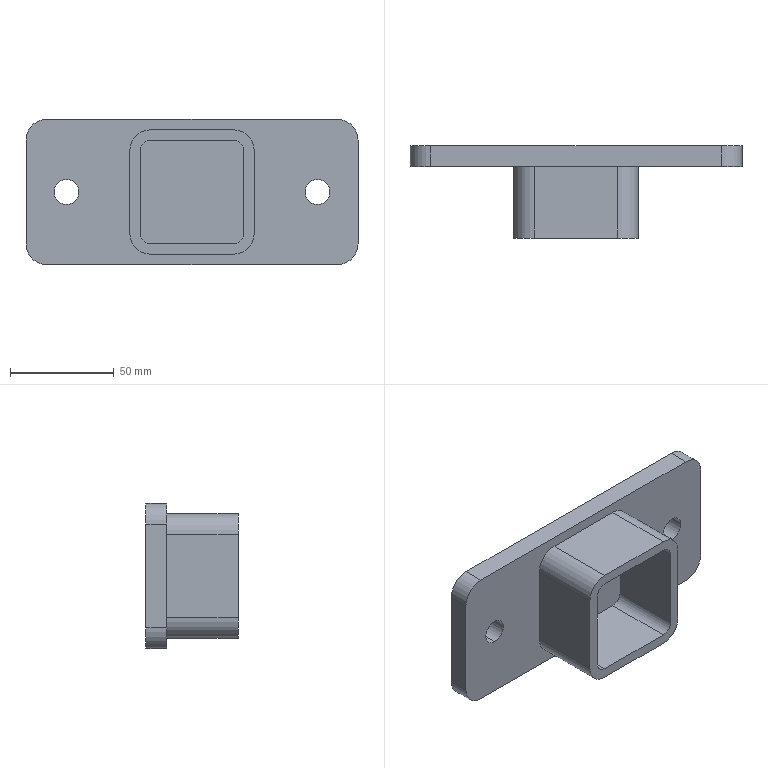Part | STEP file | BEARING_PROFILE1V11_Default<Machined> | 2 solids | 32 faces | box 160 x 44.5 x 70 mm | volume 144609 mm3 | cylinder 16 | plane 16 | commonest cylinder face diameters 20 x8 10 x4 12 x4